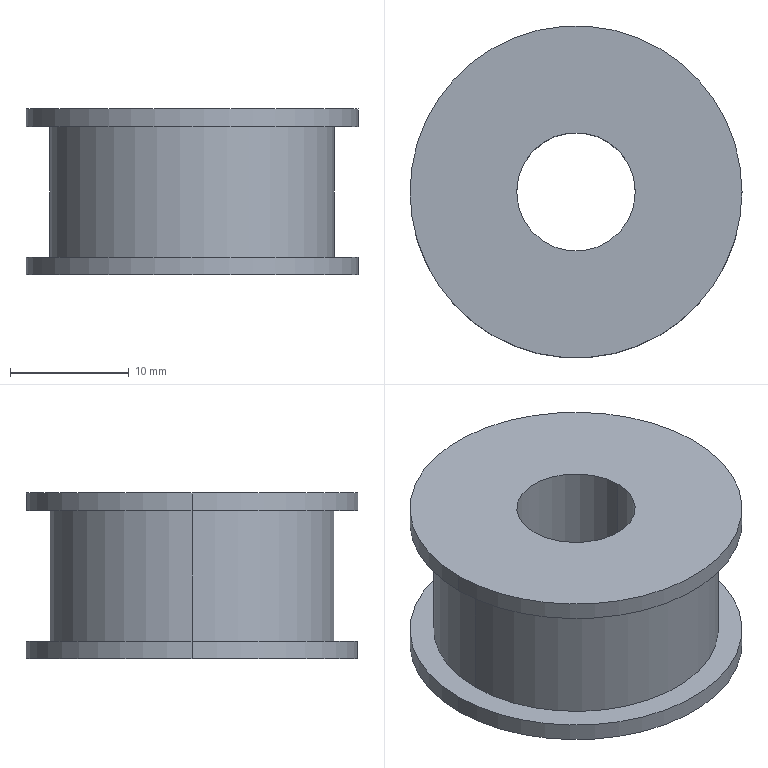Part | SolidWorks | features BaseBody 1 | 1 solid | 12 faces | box 28 x 28 x 14 mm | volume 5724 mm3 | cylinder 8 | plane 4 | commonest cylinder face diameters 28 x4 10 x2 24 x2
STEP:
#1=CARTESIAN_POINT('',(-14.,0.,1.5));
#2=VERTEX_POINT('',#1);
#3=CARTESIAN_POINT('',(14.,0.,1.5));
#4=VERTEX_POINT('',#3);
#5=CARTESIAN_POINT('',(0.,0.,1.5));
#6=DIRECTION('',(0.,0.,-1.));
#7=DIRECTION('',(-1.,0.,0.));
#8=AXIS2_PLACEMENT_3D('',#5,#6,#7);
#9=CIRCLE('',#8,14.);
#10=EDGE_CURVE('',#2,#4,#9,.T.);
#11=ORIENTED_EDGE('',*,*,#10,.T.);
#12=CARTESIAN_POINT('',(14.,0.,0.));
#13=VERTEX_POINT('',#12);
#14=CARTESIAN_POINT('',(14.,0.,1.5));
#15=DIRECTION('',(0.,0.,-1.));
#16=VECTOR('',#15,1000.);
#17=LINE('',#14,#16);
#18=EDGE_CURVE('',#4,#13,#17,.T.);
#19=ORIENTED_EDGE('',*,*,#18,.T.);
#20=CARTESIAN_POINT('',(-14.,0.,0.));
#21=VERTEX_POINT('',#20);
#22=CARTESIAN_POINT('',(0.,0.,0.));
#23=DIRECTION('',(0.,0.,1.));
#24=DIRECTION('',(-1.,0.,0.));
#25=AXIS2_PLACEMENT_3D('',#22,#23,#24);
#26=CIRCLE('',#25,14.);
#27=EDGE_CURVE('',#13,#21,#26,.T.);
#28=ORIENTED_EDGE('',*,*,#27,.T.);
#29=CARTESIAN_POINT('',(-14.,0.,1.5));
#30=DIRECTION('',(0.,0.,-1.));
#31=VECTOR('',#30,1000.);
#32=LINE('',#29,#31);
#33=EDGE_CURVE('',#2,#21,#32,.T.);
#34=ORIENTED_EDGE('',*,*,#33,.F.);
#35=EDGE_LOOP('',(#11,#19,#28,#34));
#36=FACE_OUTER_BOUND('',#35,.T.);
#37=CARTESIAN_POINT('',(0.,0.,1.5));
#38=DIRECTION('',(0.,0.,-1.));
#39=DIRECTION('',(-1.,0.,0.));
#40=AXIS2_PLACEMENT_3D('',#37,#38,#39);
#41=CYLINDRICAL_SURFACE('',#40,14.);
#42=ADVANCED_FACE('',(#36),#41,.T.);
#43=CARTESIAN_POINT('',(5.,0.,0.));
#44=VERTEX_POINT('',#43);
#45=CARTESIAN_POINT('',(-5.,0.,0.));
#46=VERTEX_POINT('',#45);
#47=CARTESIAN_POINT('',(0.,0.,0.));
#48=DIRECTION('',(0.,0.,-1.));
#49=DIRECTION('',(1.,0.,0.));
#50=AXIS2_PLACEMENT_3D('',#47,#48,#49);
#51=CIRCLE('',#50,5.);
#52=EDGE_CURVE('',#44,#46,#51,.T.);
#53=ORIENTED_EDGE('',*,*,#52,.T.);
#54=CARTESIAN_POINT('',(-5.,0.,14.));
#55=VERTEX_POINT('',#54);
#56=CARTESIAN_POINT('',(-5.,0.,-15.5));
#57=DIRECTION('',(0.,0.,1.));
#58=VECTOR('',#57,1000.);
#59=LINE('',#56,#58);
#60=EDGE_CURVE('',#46,#55,#59,.T.);
#61=ORIENTED_EDGE('',*,*,#60,.T.);
#62=CARTESIAN_POINT('',(5.,0.,14.));
#63=VERTEX_POINT('',#62);
#64=CARTESIAN_POINT('',(0.,0.,14.));
#65=DIRECTION('',(0.,0.,-1.));
#66=DIRECTION('',(1.,0.,0.));
#67=AXIS2_PLACEMENT_3D('',#64,#65,#66);
#68=CIRCLE('',#67,5.);
#69=EDGE_CURVE('',#63,#55,#68,.T.);
#70=ORIENTED_EDGE('',*,*,#69,.F.);
#71=CARTESIAN_POINT('',(5.,0.,-15.5));
#72=DIRECTION('',(0.,0.,1.));
#73=VECTOR('',#72,1000.);
#74=LINE('',#71,#73);
#75=EDGE_CURVE('',#44,#63,#74,.T.);
#76=ORIENTED_EDGE('',*,*,#75,.F.);
#77=EDGE_LOOP('',(#53,#61,#70,#76));
#78=FACE_OUTER_BOUND('',#77,.T.);
#79=CARTESIAN_POINT('',(0.,0.,-15.5));
#80=DIRECTION('',(0.,0.,1.));
#81=DIRECTION('',(1.,0.,0.));
#82=AXIS2_PLACEMENT_3D('',#79,#80,#81);
#83=CYLINDRICAL_SURFACE('',#82,5.);
#84=ADVANCED_FACE('',(#78),#83,.F.);
#85=CARTESIAN_POINT('',(-12.,0.,12.5));
#86=VERTEX_POINT('',#85);
#87=CARTESIAN_POINT('',(12.,0.,12.5));
#88=VERTEX_POINT('',#87);
#89=CARTESIAN_POINT('',(0.,0.,12.5));
#90=DIRECTION('',(0.,0.,-1.));
#91=DIRECTION('',(-1.,0.,0.));
#92=AXIS2_PLACEMENT_3D('',#89,#90,#91);
#93=CIRCLE('',#92,12.);
#94=EDGE_CURVE('',#86,#88,#93,.T.);
#95=ORIENTED_EDGE('',*,*,#94,.T.);
#96=CARTESIAN_POINT('',(12.,0.,1.5));
#97=VERTEX_POINT('',#96);
#98=CARTESIAN_POINT('',(12.,0.,12.5));
#99=DIRECTION('',(0.,0.,-1.));
#100=VECTOR('',#99,1000.);
#101=LINE('',#98,#100);
#102=EDGE_CURVE('',#88,#97,#101,.T.);
#103=ORIENTED_EDGE('',*,*,#102,.T.);
#104=CARTESIAN_POINT('',(-12.,0.,1.5));
#105=VERTEX_POINT('',#104);
#106=CARTESIAN_POINT('',(0.,0.,1.5));
#107=DIRECTION('',(0.,0.,-1.));
#108=DIRECTION('',(-1.,0.,0.));
#109=AXIS2_PLACEMENT_3D('',#106,#107,#108);
#110=CIRCLE('',#109,12.);
#111=EDGE_CURVE('',#105,#97,#110,.T.);
#112=ORIENTED_EDGE('',*,*,#111,.F.);
#113=CARTESIAN_POINT('',(-12.,0.,12.5));
#114=DIRECTION('',(0.,0.,-1.));
#115=VECTOR('',#114,1000.);
#116=LINE('',#113,#115);
#117=EDGE_CURVE('',#86,#105,#116,.T.);
#118=ORIENTED_EDGE('',*,*,#117,.F.);
#119=EDGE_LOOP('',(#95,#103,#112,#118));
#120=FACE_OUTER_BOUND('',#119,.T.);
#121=CARTESIAN_POINT('',(0.,0.,12.5));
#122=DIRECTION('',(0.,0.,-1.));
#123=DIRECTION('',(-1.,0.,0.));
#124=AXIS2_PLACEMENT_3D('',#121,#122,#123);
#125=CYLINDRICAL_SURFACE('',#124,12.);
#126=ADVANCED_FACE('',(#120),#125,.T.);
#127=CARTESIAN_POINT('',(14.,0.,14.));
#128=VERTEX_POINT('',#127);
#129=CARTESIAN_POINT('',(-14.,0.,14.));
#130=VERTEX_POINT('',#129);
#131=CARTESIAN_POINT('',(0.,0.,14.));
#132=DIRECTION('',(0.,0.,1.));
#133=DIRECTION('',(-1.,0.,0.));
#134=AXIS2_PLACEMENT_3D('',#131,#132,#133);
#135=CIRCLE('',#134,14.);
#136=EDGE_CURVE('',#128,#130,#135,.T.);
#137=ORIENTED_EDGE('',*,*,#136,.F.);
#138=CARTESIAN_POINT('',(14.,0.,12.5));
#139=VERTEX_POINT('',#138);
#140=CARTESIAN_POINT('',(14.,0.,14.));
#141=DIRECTION('',(0.,0.,-1.));
#142=VECTOR('',#141,1000.);
#143=LINE('',#140,#142);
#144=EDGE_CURVE('',#128,#139,#143,.T.);
#145=ORIENTED_EDGE('',*,*,#144,.T.);
#146=CARTESIAN_POINT('',(-14.,0.,12.5));
#147=VERTEX_POINT('',#146);
#148=CARTESIAN_POINT('',(0.,0.,12.5));
#149=DIRECTION('',(0.,0.,1.));
#150=DIRECTION('',(-1.,0.,0.));
#151=AXIS2_PLACEMENT_3D('',#148,#149,#150);
#152=CIRCLE('',#151,14.);
#153=EDGE_CURVE('',#139,#147,#152,.T.);
#154=ORIENTED_EDGE('',*,*,#153,.T.);
#155=CARTESIAN_POINT('',(-14.,0.,14.));
#156=DIRECTION('',(0.,0.,-1.));
#157=VECTOR('',#156,1000.);
#158=LINE('',#155,#157);
#159=EDGE_CURVE('',#130,#147,#158,.T.);
#160=ORIENTED_EDGE('',*,*,#159,.F.);
#161=EDGE_LOOP('',(#137,#145,#154,#160));
#162=FACE_OUTER_BOUND('',#161,.T.);
#163=CARTESIAN_POINT('',(0.,0.,14.));
#164=DIRECTION('',(0.,0.,-1.));
#165=DIRECTION('',(-1.,0.,0.));
#166=AXIS2_PLACEMENT_3D('',#163,#164,#165);
#167=CYLINDRICAL_SURFACE('',#166,14.);
#168=ADVANCED_FACE('',(#162),#167,.T.);
#169=CARTESIAN_POINT('',(0.,0.,0.));
#170=DIRECTION('',(0.,0.,1.));
#171=DIRECTION('',(-1.,0.,0.));
#172=AXIS2_PLACEMENT_3D('',#169,#170,#171);
#173=CIRCLE('',#172,14.);
#174=EDGE_CURVE('',#21,#13,#173,.T.);
#175=ORIENTED_EDGE('',*,*,#174,.F.);
#176=ORIENTED_EDGE('',*,*,#27,.F.);
#177=EDGE_LOOP('',(#175,#176));
#178=FACE_OUTER_BOUND('',#177,.T.);
#179=ORIENTED_EDGE('',*,*,#52,.F.);
#180=CARTESIAN_POINT('',(0.,0.,0.));
#181=DIRECTION('',(0.,0.,-1.));
#182=DIRECTION('',(1.,0.,0.));
#183=AXIS2_PLACEMENT_3D('',#180,#181,#182);
#184=CIRCLE('',#183,5.);
#185=EDGE_CURVE('',#46,#44,#184,.T.);
#186=ORIENTED_EDGE('',*,*,#185,.F.);
#187=EDGE_LOOP('',(#179,#186));
#188=FACE_BOUND('',#187,.T.);
#189=CARTESIAN_POINT('',(0.,0.,0.));
#190=DIRECTION('',(0.,0.,1.));
#191=DIRECTION('',(1.,0.,0.));
#192=AXIS2_PLACEMENT_3D('',#189,#190,#191);
#193=PLANE('',#192);
#194=ADVANCED_FACE('',(#178,#188),#193,.F.);
#195=ORIENTED_EDGE('',*,*,#18,.F.);
#196=CARTESIAN_POINT('',(0.,0.,1.5));
#197=DIRECTION('',(0.,0.,-1.));
#198=DIRECTION('',(-1.,0.,0.));
#199=AXIS2_PLACEMENT_3D('',#196,#197,#198);
#200=CIRCLE('',#199,14.);
#201=EDGE_CURVE('',#4,#2,#200,.T.);
#202=ORIENTED_EDGE('',*,*,#201,.T.);
#203=ORIENTED_EDGE('',*,*,#33,.T.);
#204=ORIENTED_EDGE('',*,*,#174,.T.);
#205=EDGE_LOOP('',(#195,#202,#203,#204));
#206=FACE_OUTER_BOUND('',#205,.T.);
#207=CARTESIAN_POINT('',(0.,0.,1.5));
#208=DIRECTION('',(0.,0.,-1.));
#209=DIRECTION('',(-1.,0.,0.));
#210=AXIS2_PLACEMENT_3D('',#207,#208,#209);
#211=CYLINDRICAL_SURFACE('',#210,14.);
#212=ADVANCED_FACE('',(#206),#211,.T.);
#213=ORIENTED_EDGE('',*,*,#60,.F.);
#214=ORIENTED_EDGE('',*,*,#185,.T.);
#215=ORIENTED_EDGE('',*,*,#75,.T.);
#216=CARTESIAN_POINT('',(0.,0.,14.));
#217=DIRECTION('',(0.,0.,-1.));
#218=DIRECTION('',(1.,0.,0.));
#219=AXIS2_PLACEMENT_3D('',#216,#217,#218);
#220=CIRCLE('',#219,5.);
#221=EDGE_CURVE('',#55,#63,#220,.T.);
#222=ORIENTED_EDGE('',*,*,#221,.F.);
#223=EDGE_LOOP('',(#213,#214,#215,#222));
#224=FACE_OUTER_BOUND('',#223,.T.);
#225=CARTESIAN_POINT('',(0.,0.,-15.5));
#226=DIRECTION('',(0.,0.,1.));
#227=DIRECTION('',(1.,0.,0.));
#228=AXIS2_PLACEMENT_3D('',#225,#226,#227);
#229=CYLINDRICAL_SURFACE('',#228,5.);
#230=ADVANCED_FACE('',(#224),#229,.F.);
#231=ORIENTED_EDGE('',*,*,#10,.F.);
#232=ORIENTED_EDGE('',*,*,#201,.F.);
#233=EDGE_LOOP('',(#231,#232));
#234=FACE_OUTER_BOUND('',#233,.T.);
#235=ORIENTED_EDGE('',*,*,#111,.T.);
#236=CARTESIAN_POINT('',(0.,0.,1.5));
#237=DIRECTION('',(0.,0.,-1.));
#238=DIRECTION('',(-1.,0.,0.));
#239=AXIS2_PLACEMENT_3D('',#236,#237,#238);
#240=CIRCLE('',#239,12.);
#241=EDGE_CURVE('',#97,#105,#240,.T.);
#242=ORIENTED_EDGE('',*,*,#241,.T.);
#243=EDGE_LOOP('',(#235,#242));
#244=FACE_BOUND('',#243,.T.);
#245=CARTESIAN_POINT('',(0.,0.,1.5));
#246=DIRECTION('',(0.,0.,1.));
#247=DIRECTION('',(1.,0.,0.));
#248=AXIS2_PLACEMENT_3D('',#245,#246,#247);
#249=PLANE('',#248);
#250=ADVANCED_FACE('',(#234,#244),#249,.T.);
#251=CARTESIAN_POINT('',(0.,0.,14.));
#252=DIRECTION('',(0.,0.,1.));
#253=DIRECTION('',(-1.,0.,0.));
#254=AXIS2_PLACEMENT_3D('',#251,#252,#253);
#255=CIRCLE('',#254,14.);
#256=EDGE_CURVE('',#130,#128,#255,.T.);
#257=ORIENTED_EDGE('',*,*,#256,.T.);
#258=ORIENTED_EDGE('',*,*,#136,.T.);
#259=EDGE_LOOP('',(#257,#258));
#260=FACE_OUTER_BOUND('',#259,.T.);
#261=ORIENTED_EDGE('',*,*,#69,.T.);
#262=ORIENTED_EDGE('',*,*,#221,.T.);
#263=EDGE_LOOP('',(#261,#262));
#264=FACE_BOUND('',#263,.T.);
#265=CARTESIAN_POINT('',(0.,0.,14.));
#266=DIRECTION('',(0.,0.,1.));
#267=DIRECTION('',(1.,0.,0.));
#268=AXIS2_PLACEMENT_3D('',#265,#266,#267);
#269=PLANE('',#268);
#270=ADVANCED_FACE('',(#260,#264),#269,.T.);
#271=ORIENTED_EDGE('',*,*,#102,.F.);
#272=CARTESIAN_POINT('',(0.,0.,12.5));
#273=DIRECTION('',(0.,0.,-1.));
#274=DIRECTION('',(-1.,0.,0.));
#275=AXIS2_PLACEMENT_3D('',#272,#273,#274);
#276=CIRCLE('',#275,12.);
#277=EDGE_CURVE('',#88,#86,#276,.T.);
#278=ORIENTED_EDGE('',*,*,#277,.T.);
#279=ORIENTED_EDGE('',*,*,#117,.T.);
#280=ORIENTED_EDGE('',*,*,#241,.F.);
#281=EDGE_LOOP('',(#271,#278,#279,#280));
#282=FACE_OUTER_BOUND('',#281,.T.);
#283=CARTESIAN_POINT('',(0.,0.,12.5));
#284=DIRECTION('',(0.,0.,-1.));
#285=DIRECTION('',(-1.,0.,0.));
#286=AXIS2_PLACEMENT_3D('',#283,#284,#285);
#287=CYLINDRICAL_SURFACE('',#286,12.);
#288=ADVANCED_FACE('',(#282),#287,.T.);
#289=ORIENTED_EDGE('',*,*,#144,.F.);
#290=ORIENTED_EDGE('',*,*,#256,.F.);
#291=ORIENTED_EDGE('',*,*,#159,.T.);
#292=CARTESIAN_POINT('',(0.,0.,12.5));
#293=DIRECTION('',(0.,0.,1.));
#294=DIRECTION('',(-1.,0.,0.));
#295=AXIS2_PLACEMENT_3D('',#292,#293,#294);
#296=CIRCLE('',#295,14.);
#297=EDGE_CURVE('',#147,#139,#296,.T.);
#298=ORIENTED_EDGE('',*,*,#297,.T.);
#299=EDGE_LOOP('',(#289,#290,#291,#298));
#300=FACE_OUTER_BOUND('',#299,.T.);
#301=CARTESIAN_POINT('',(0.,0.,14.));
#302=DIRECTION('',(0.,0.,-1.));
#303=DIRECTION('',(-1.,0.,0.));
#304=AXIS2_PLACEMENT_3D('',#301,#302,#303);
#305=CYLINDRICAL_SURFACE('',#304,14.);
#306=ADVANCED_FACE('',(#300),#305,.T.);
#307=ORIENTED_EDGE('',*,*,#297,.F.);
#308=ORIENTED_EDGE('',*,*,#153,.F.);
#309=EDGE_LOOP('',(#307,#308));
#310=FACE_OUTER_BOUND('',#309,.T.);
#311=ORIENTED_EDGE('',*,*,#94,.F.);
#312=ORIENTED_EDGE('',*,*,#277,.F.);
#313=EDGE_LOOP('',(#311,#312));
#314=FACE_BOUND('',#313,.T.);
#315=CARTESIAN_POINT('',(0.,0.,12.5));
#316=DIRECTION('',(0.,0.,1.));
#317=DIRECTION('',(1.,0.,0.));
#318=AXIS2_PLACEMENT_3D('',#315,#316,#317);
#319=PLANE('',#318);
#320=ADVANCED_FACE('',(#310,#314),#319,.F.);
#321=CLOSED_SHELL('',(#42,#84,#126,#168,#194,#212,#230,#250,#270,#288,#306,#320));
#322=MANIFOLD_SOLID_BREP('',#321);
#323=CARTESIAN_POINT('',(0.,0.,0.));
#324=DIRECTION('',(0.,0.,1.));
#325=DIRECTION('',(1.,0.,0.));
#326=AXIS2_PLACEMENT_3D('',#323,#324,#325);
#327=(LENGTH_UNIT()NAMED_UNIT(*)SI_UNIT(.MILLI.,.METRE.));
#328=UNCERTAINTY_MEASURE_WITH_UNIT(LENGTH_MEASURE(0.00001),#327,'','');
#329=(NAMED_UNIT(*)PLANE_ANGLE_UNIT()SI_UNIT($,.RADIAN.));
#330=(NAMED_UNIT(*)SI_UNIT($,.STERADIAN.)SOLID_ANGLE_UNIT());
#331=(GEOMETRIC_REPRESENTATION_CONTEXT(3)GLOBAL_UNCERTAINTY_ASSIGNED_CONTEXT((#328))GLOBAL_UNIT_ASSIGNED_CONTEXT((#327,#329,#330))REPRESENTATION_CONTEXT('',''));
#332=ADVANCED_BREP_SHAPE_REPRESENTATION('',(#322,#326),#331);